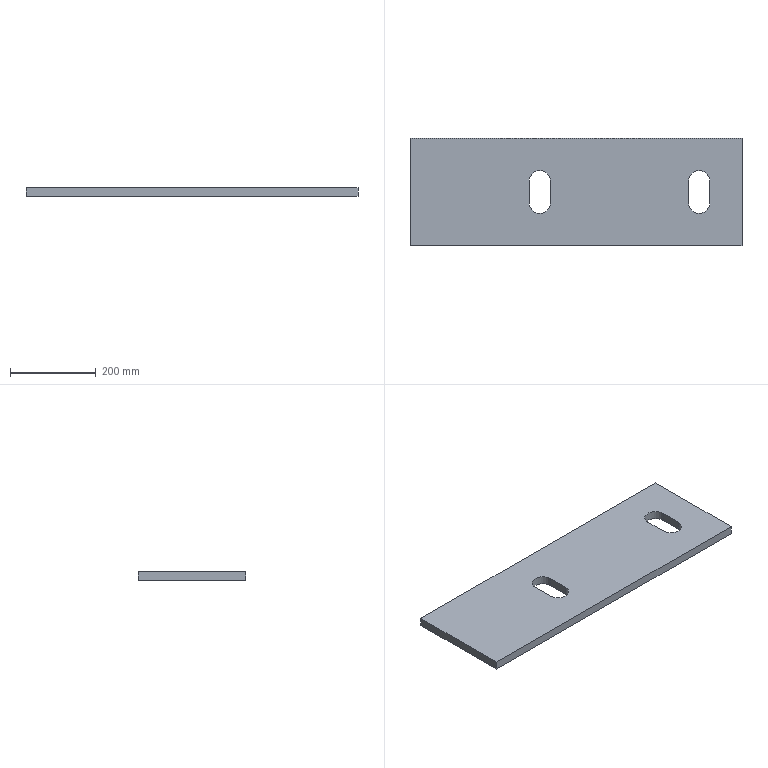Part | SolidWorks | features Extrusion 1 | 1 solid | 14 faces | box 775.098 x 250 x 20 mm | volume 3696953 mm3 | plane 10 | cylinder 4 | commonest cylinder face diameters 50 x4
STEP:
#1=CARTESIAN_POINT('',(13593.233,4558.16,20.));
#2=VERTEX_POINT('',#1);
#3=CARTESIAN_POINT('',(13543.233,4558.16,20.));
#4=VERTEX_POINT('',#3);
#5=CARTESIAN_POINT('',(13568.233,4558.16,20.));
#6=DIRECTION('',(0.,0.,1.));
#7=DIRECTION('',(1.,0.,0.));
#8=AXIS2_PLACEMENT_3D('',#5,#6,#7);
#9=CIRCLE('',#8,25.);
#10=EDGE_CURVE('',#2,#4,#9,.T.);
#11=ORIENTED_EDGE('',*,*,#10,.F.);
#12=CARTESIAN_POINT('',(13593.233,4508.16,20.));
#13=VERTEX_POINT('',#12);
#14=CARTESIAN_POINT('',(13593.233,4558.16,20.));
#15=DIRECTION('',(0.,1.,0.));
#16=VECTOR('',#15,1000.);
#17=LINE('',#14,#16);
#18=EDGE_CURVE('',#13,#2,#17,.T.);
#19=ORIENTED_EDGE('',*,*,#18,.F.);
#20=CARTESIAN_POINT('',(13543.233,4508.16,20.));
#21=VERTEX_POINT('',#20);
#22=CARTESIAN_POINT('',(13568.233,4508.16,20.));
#23=DIRECTION('',(0.,0.,1.));
#24=DIRECTION('',(1.,0.,0.));
#25=AXIS2_PLACEMENT_3D('',#22,#23,#24);
#26=CIRCLE('',#25,25.);
#27=EDGE_CURVE('',#21,#13,#26,.T.);
#28=ORIENTED_EDGE('',*,*,#27,.F.);
#29=CARTESIAN_POINT('',(13543.233,4558.16,20.));
#30=DIRECTION('',(0.,-1.,0.));
#31=VECTOR('',#30,1000.);
#32=LINE('',#29,#31);
#33=EDGE_CURVE('',#4,#21,#32,.T.);
#34=ORIENTED_EDGE('',*,*,#33,.F.);
#35=EDGE_LOOP('',(#11,#19,#28,#34));
#36=FACE_BOUND('',#35,.T.);
#37=CARTESIAN_POINT('',(14040.331,4658.16,20.));
#38=VERTEX_POINT('',#37);
#39=CARTESIAN_POINT('',(13265.233,4658.16,20.));
#40=VERTEX_POINT('',#39);
#41=CARTESIAN_POINT('',(13265.233,4658.16,20.));
#42=DIRECTION('',(-1.,0.,0.));
#43=VECTOR('',#42,1000.);
#44=LINE('',#41,#43);
#45=EDGE_CURVE('',#38,#40,#44,.T.);
#46=ORIENTED_EDGE('',*,*,#45,.T.);
#47=CARTESIAN_POINT('',(13265.233,4408.16,20.));
#48=VERTEX_POINT('',#47);
#49=CARTESIAN_POINT('',(13265.233,4658.16,20.));
#50=DIRECTION('',(0.,-1.,0.));
#51=VECTOR('',#50,1000.);
#52=LINE('',#49,#51);
#53=EDGE_CURVE('',#40,#48,#52,.T.);
#54=ORIENTED_EDGE('',*,*,#53,.T.);
#55=CARTESIAN_POINT('',(14040.331,4408.16,20.));
#56=VERTEX_POINT('',#55);
#57=CARTESIAN_POINT('',(13265.233,4408.16,20.));
#58=DIRECTION('',(1.,0.,0.));
#59=VECTOR('',#58,1000.);
#60=LINE('',#57,#59);
#61=EDGE_CURVE('',#48,#56,#60,.T.);
#62=ORIENTED_EDGE('',*,*,#61,.T.);
#63=CARTESIAN_POINT('',(14040.331,4658.16,20.));
#64=DIRECTION('',(0.,1.,0.));
#65=VECTOR('',#64,1000.);
#66=LINE('',#63,#65);
#67=EDGE_CURVE('',#56,#38,#66,.T.);
#68=ORIENTED_EDGE('',*,*,#67,.T.);
#69=EDGE_LOOP('',(#46,#54,#62,#68));
#70=FACE_OUTER_BOUND('',#69,.T.);
#71=CARTESIAN_POINT('',(13965.331,4558.16,20.));
#72=VERTEX_POINT('',#71);
#73=CARTESIAN_POINT('',(13915.331,4558.16,20.));
#74=VERTEX_POINT('',#73);
#75=CARTESIAN_POINT('',(13940.331,4558.16,20.));
#76=DIRECTION('',(0.,0.,1.));
#77=DIRECTION('',(1.,0.,0.));
#78=AXIS2_PLACEMENT_3D('',#75,#76,#77);
#79=CIRCLE('',#78,25.);
#80=EDGE_CURVE('',#72,#74,#79,.T.);
#81=ORIENTED_EDGE('',*,*,#80,.F.);
#82=CARTESIAN_POINT('',(13965.331,4508.16,20.));
#83=VERTEX_POINT('',#82);
#84=CARTESIAN_POINT('',(13965.331,4558.16,20.));
#85=DIRECTION('',(0.,1.,0.));
#86=VECTOR('',#85,1000.);
#87=LINE('',#84,#86);
#88=EDGE_CURVE('',#83,#72,#87,.T.);
#89=ORIENTED_EDGE('',*,*,#88,.F.);
#90=CARTESIAN_POINT('',(13915.331,4508.16,20.));
#91=VERTEX_POINT('',#90);
#92=CARTESIAN_POINT('',(13940.331,4508.16,20.));
#93=DIRECTION('',(0.,0.,1.));
#94=DIRECTION('',(1.,0.,0.));
#95=AXIS2_PLACEMENT_3D('',#92,#93,#94);
#96=CIRCLE('',#95,25.);
#97=EDGE_CURVE('',#91,#83,#96,.T.);
#98=ORIENTED_EDGE('',*,*,#97,.F.);
#99=CARTESIAN_POINT('',(13915.331,4558.16,20.));
#100=DIRECTION('',(0.,-1.,0.));
#101=VECTOR('',#100,1000.);
#102=LINE('',#99,#101);
#103=EDGE_CURVE('',#74,#91,#102,.T.);
#104=ORIENTED_EDGE('',*,*,#103,.F.);
#105=EDGE_LOOP('',(#81,#89,#98,#104));
#106=FACE_BOUND('',#105,.T.);
#107=CARTESIAN_POINT('',(0.,0.,20.));
#108=DIRECTION('',(0.,0.,-1.));
#109=DIRECTION('',(-1.,0.,0.));
#110=AXIS2_PLACEMENT_3D('',#107,#108,#109);
#111=PLANE('',#110);
#112=ADVANCED_FACE('',(#36,#70,#106),#111,.F.);
#113=CARTESIAN_POINT('',(14040.331,4658.16,0.));
#114=VERTEX_POINT('',#113);
#115=CARTESIAN_POINT('',(13265.233,4658.16,0.));
#116=VERTEX_POINT('',#115);
#117=CARTESIAN_POINT('',(13265.233,4658.16,0.));
#118=DIRECTION('',(-1.,0.,0.));
#119=VECTOR('',#118,1000.);
#120=LINE('',#117,#119);
#121=EDGE_CURVE('',#114,#116,#120,.T.);
#122=ORIENTED_EDGE('',*,*,#121,.F.);
#123=CARTESIAN_POINT('',(14040.331,4408.16,0.));
#124=VERTEX_POINT('',#123);
#125=CARTESIAN_POINT('',(14040.331,4658.16,0.));
#126=DIRECTION('',(0.,1.,0.));
#127=VECTOR('',#126,1000.);
#128=LINE('',#125,#127);
#129=EDGE_CURVE('',#124,#114,#128,.T.);
#130=ORIENTED_EDGE('',*,*,#129,.F.);
#131=CARTESIAN_POINT('',(13265.233,4408.16,0.));
#132=VERTEX_POINT('',#131);
#133=CARTESIAN_POINT('',(13265.233,4408.16,0.));
#134=DIRECTION('',(1.,0.,0.));
#135=VECTOR('',#134,1000.);
#136=LINE('',#133,#135);
#137=EDGE_CURVE('',#132,#124,#136,.T.);
#138=ORIENTED_EDGE('',*,*,#137,.F.);
#139=CARTESIAN_POINT('',(13265.233,4658.16,0.));
#140=DIRECTION('',(0.,-1.,0.));
#141=VECTOR('',#140,1000.);
#142=LINE('',#139,#141);
#143=EDGE_CURVE('',#116,#132,#142,.T.);
#144=ORIENTED_EDGE('',*,*,#143,.F.);
#145=EDGE_LOOP('',(#122,#130,#138,#144));
#146=FACE_OUTER_BOUND('',#145,.T.);
#147=CARTESIAN_POINT('',(13593.233,4508.16,0.));
#148=VERTEX_POINT('',#147);
#149=CARTESIAN_POINT('',(13593.233,4558.16,0.));
#150=VERTEX_POINT('',#149);
#151=CARTESIAN_POINT('',(13593.233,4558.16,0.));
#152=DIRECTION('',(0.,1.,0.));
#153=VECTOR('',#152,1000.);
#154=LINE('',#151,#153);
#155=EDGE_CURVE('',#148,#150,#154,.T.);
#156=ORIENTED_EDGE('',*,*,#155,.T.);
#157=CARTESIAN_POINT('',(13543.233,4558.16,0.));
#158=VERTEX_POINT('',#157);
#159=CARTESIAN_POINT('',(13568.233,4558.16,0.));
#160=DIRECTION('',(0.,0.,1.));
#161=DIRECTION('',(1.,0.,0.));
#162=AXIS2_PLACEMENT_3D('',#159,#160,#161);
#163=CIRCLE('',#162,25.);
#164=EDGE_CURVE('',#150,#158,#163,.T.);
#165=ORIENTED_EDGE('',*,*,#164,.T.);
#166=CARTESIAN_POINT('',(13543.233,4508.16,0.));
#167=VERTEX_POINT('',#166);
#168=CARTESIAN_POINT('',(13543.233,4558.16,0.));
#169=DIRECTION('',(0.,-1.,0.));
#170=VECTOR('',#169,1000.);
#171=LINE('',#168,#170);
#172=EDGE_CURVE('',#158,#167,#171,.T.);
#173=ORIENTED_EDGE('',*,*,#172,.T.);
#174=CARTESIAN_POINT('',(13568.233,4508.16,0.));
#175=DIRECTION('',(0.,0.,1.));
#176=DIRECTION('',(1.,0.,0.));
#177=AXIS2_PLACEMENT_3D('',#174,#175,#176);
#178=CIRCLE('',#177,25.);
#179=EDGE_CURVE('',#167,#148,#178,.T.);
#180=ORIENTED_EDGE('',*,*,#179,.T.);
#181=EDGE_LOOP('',(#156,#165,#173,#180));
#182=FACE_BOUND('',#181,.T.);
#183=CARTESIAN_POINT('',(13965.331,4508.16,0.));
#184=VERTEX_POINT('',#183);
#185=CARTESIAN_POINT('',(13965.331,4558.16,0.));
#186=VERTEX_POINT('',#185);
#187=CARTESIAN_POINT('',(13965.331,4558.16,0.));
#188=DIRECTION('',(0.,1.,0.));
#189=VECTOR('',#188,1000.);
#190=LINE('',#187,#189);
#191=EDGE_CURVE('',#184,#186,#190,.T.);
#192=ORIENTED_EDGE('',*,*,#191,.T.);
#193=CARTESIAN_POINT('',(13915.331,4558.16,0.));
#194=VERTEX_POINT('',#193);
#195=CARTESIAN_POINT('',(13940.331,4558.16,0.));
#196=DIRECTION('',(0.,0.,1.));
#197=DIRECTION('',(1.,0.,0.));
#198=AXIS2_PLACEMENT_3D('',#195,#196,#197);
#199=CIRCLE('',#198,25.);
#200=EDGE_CURVE('',#186,#194,#199,.T.);
#201=ORIENTED_EDGE('',*,*,#200,.T.);
#202=CARTESIAN_POINT('',(13915.331,4508.16,0.));
#203=VERTEX_POINT('',#202);
#204=CARTESIAN_POINT('',(13915.331,4558.16,0.));
#205=DIRECTION('',(0.,-1.,0.));
#206=VECTOR('',#205,1000.);
#207=LINE('',#204,#206);
#208=EDGE_CURVE('',#194,#203,#207,.T.);
#209=ORIENTED_EDGE('',*,*,#208,.T.);
#210=CARTESIAN_POINT('',(13940.331,4508.16,0.));
#211=DIRECTION('',(0.,0.,1.));
#212=DIRECTION('',(1.,0.,0.));
#213=AXIS2_PLACEMENT_3D('',#210,#211,#212);
#214=CIRCLE('',#213,25.);
#215=EDGE_CURVE('',#203,#184,#214,.T.);
#216=ORIENTED_EDGE('',*,*,#215,.T.);
#217=EDGE_LOOP('',(#192,#201,#209,#216));
#218=FACE_BOUND('',#217,.T.);
#219=CARTESIAN_POINT('',(0.,0.,0.));
#220=DIRECTION('',(0.,0.,-1.));
#221=DIRECTION('',(-1.,0.,0.));
#222=AXIS2_PLACEMENT_3D('',#219,#220,#221);
#223=PLANE('',#222);
#224=ADVANCED_FACE('',(#146,#182,#218),#223,.T.);
#225=ORIENTED_EDGE('',*,*,#121,.T.);
#226=CARTESIAN_POINT('',(13265.233,4658.16,20.));
#227=DIRECTION('',(0.,0.,-1.));
#228=VECTOR('',#227,1000.);
#229=LINE('',#226,#228);
#230=EDGE_CURVE('',#40,#116,#229,.T.);
#231=ORIENTED_EDGE('',*,*,#230,.F.);
#232=ORIENTED_EDGE('',*,*,#45,.F.);
#233=CARTESIAN_POINT('',(14040.331,4658.16,20.));
#234=DIRECTION('',(0.,0.,-1.));
#235=VECTOR('',#234,1000.);
#236=LINE('',#233,#235);
#237=EDGE_CURVE('',#38,#114,#236,.T.);
#238=ORIENTED_EDGE('',*,*,#237,.T.);
#239=EDGE_LOOP('',(#225,#231,#232,#238));
#240=FACE_OUTER_BOUND('',#239,.T.);
#241=CARTESIAN_POINT('',(13265.233,4658.16,20.));
#242=DIRECTION('',(0.,-1.,0.));
#243=DIRECTION('',(0.,0.,-1.));
#244=AXIS2_PLACEMENT_3D('',#241,#242,#243);
#245=PLANE('',#244);
#246=ADVANCED_FACE('',(#240),#245,.F.);
#247=ORIENTED_EDGE('',*,*,#143,.T.);
#248=CARTESIAN_POINT('',(13265.233,4408.16,20.));
#249=DIRECTION('',(0.,0.,-1.));
#250=VECTOR('',#249,1000.);
#251=LINE('',#248,#250);
#252=EDGE_CURVE('',#48,#132,#251,.T.);
#253=ORIENTED_EDGE('',*,*,#252,.F.);
#254=ORIENTED_EDGE('',*,*,#53,.F.);
#255=ORIENTED_EDGE('',*,*,#230,.T.);
#256=EDGE_LOOP('',(#247,#253,#254,#255));
#257=FACE_OUTER_BOUND('',#256,.T.);
#258=CARTESIAN_POINT('',(13265.233,4658.16,20.));
#259=DIRECTION('',(1.,0.,0.));
#260=DIRECTION('',(0.,1.,0.));
#261=AXIS2_PLACEMENT_3D('',#258,#259,#260);
#262=PLANE('',#261);
#263=ADVANCED_FACE('',(#257),#262,.F.);
#264=ORIENTED_EDGE('',*,*,#137,.T.);
#265=CARTESIAN_POINT('',(14040.331,4408.16,20.));
#266=DIRECTION('',(0.,0.,-1.));
#267=VECTOR('',#266,1000.);
#268=LINE('',#265,#267);
#269=EDGE_CURVE('',#56,#124,#268,.T.);
#270=ORIENTED_EDGE('',*,*,#269,.F.);
#271=ORIENTED_EDGE('',*,*,#61,.F.);
#272=ORIENTED_EDGE('',*,*,#252,.T.);
#273=EDGE_LOOP('',(#264,#270,#271,#272));
#274=FACE_OUTER_BOUND('',#273,.T.);
#275=CARTESIAN_POINT('',(13265.233,4408.16,20.));
#276=DIRECTION('',(0.,1.,0.));
#277=DIRECTION('',(0.,0.,1.));
#278=AXIS2_PLACEMENT_3D('',#275,#276,#277);
#279=PLANE('',#278);
#280=ADVANCED_FACE('',(#274),#279,.F.);
#281=ORIENTED_EDGE('',*,*,#129,.T.);
#282=ORIENTED_EDGE('',*,*,#237,.F.);
#283=ORIENTED_EDGE('',*,*,#67,.F.);
#284=ORIENTED_EDGE('',*,*,#269,.T.);
#285=EDGE_LOOP('',(#281,#282,#283,#284));
#286=FACE_OUTER_BOUND('',#285,.T.);
#287=CARTESIAN_POINT('',(14040.331,4658.16,20.));
#288=DIRECTION('',(-1.,0.,0.));
#289=DIRECTION('',(0.,0.,1.));
#290=AXIS2_PLACEMENT_3D('',#287,#288,#289);
#291=PLANE('',#290);
#292=ADVANCED_FACE('',(#286),#291,.F.);
#293=ORIENTED_EDGE('',*,*,#164,.F.);
#294=CARTESIAN_POINT('',(13593.233,4558.16,20.));
#295=DIRECTION('',(0.,0.,-1.));
#296=VECTOR('',#295,1000.);
#297=LINE('',#294,#296);
#298=EDGE_CURVE('',#2,#150,#297,.T.);
#299=ORIENTED_EDGE('',*,*,#298,.F.);
#300=ORIENTED_EDGE('',*,*,#10,.T.);
#301=CARTESIAN_POINT('',(13543.233,4558.16,20.));
#302=DIRECTION('',(0.,0.,-1.));
#303=VECTOR('',#302,1000.);
#304=LINE('',#301,#303);
#305=EDGE_CURVE('',#4,#158,#304,.T.);
#306=ORIENTED_EDGE('',*,*,#305,.T.);
#307=EDGE_LOOP('',(#293,#299,#300,#306));
#308=FACE_OUTER_BOUND('',#307,.T.);
#309=CARTESIAN_POINT('',(13568.233,4558.16,20.));
#310=DIRECTION('',(0.,0.,-1.));
#311=DIRECTION('',(-1.,0.,0.));
#312=AXIS2_PLACEMENT_3D('',#309,#310,#311);
#313=CYLINDRICAL_SURFACE('',#312,25.);
#314=ADVANCED_FACE('',(#308),#313,.F.);
#315=ORIENTED_EDGE('',*,*,#172,.F.);
#316=ORIENTED_EDGE('',*,*,#305,.F.);
#317=ORIENTED_EDGE('',*,*,#33,.T.);
#318=CARTESIAN_POINT('',(13543.233,4508.16,20.));
#319=DIRECTION('',(0.,0.,-1.));
#320=VECTOR('',#319,1000.);
#321=LINE('',#318,#320);
#322=EDGE_CURVE('',#21,#167,#321,.T.);
#323=ORIENTED_EDGE('',*,*,#322,.T.);
#324=EDGE_LOOP('',(#315,#316,#317,#323));
#325=FACE_OUTER_BOUND('',#324,.T.);
#326=CARTESIAN_POINT('',(13543.233,4558.16,20.));
#327=DIRECTION('',(1.,0.,0.));
#328=DIRECTION('',(0.,0.,-1.));
#329=AXIS2_PLACEMENT_3D('',#326,#327,#328);
#330=PLANE('',#329);
#331=ADVANCED_FACE('',(#325),#330,.T.);
#332=ORIENTED_EDGE('',*,*,#179,.F.);
#333=ORIENTED_EDGE('',*,*,#322,.F.);
#334=ORIENTED_EDGE('',*,*,#27,.T.);
#335=CARTESIAN_POINT('',(13593.233,4508.16,20.));
#336=DIRECTION('',(0.,0.,-1.));
#337=VECTOR('',#336,1000.);
#338=LINE('',#335,#337);
#339=EDGE_CURVE('',#13,#148,#338,.T.);
#340=ORIENTED_EDGE('',*,*,#339,.T.);
#341=EDGE_LOOP('',(#332,#333,#334,#340));
#342=FACE_OUTER_BOUND('',#341,.T.);
#343=CARTESIAN_POINT('',(13568.233,4508.16,20.));
#344=DIRECTION('',(0.,0.,-1.));
#345=DIRECTION('',(-1.,0.,0.));
#346=AXIS2_PLACEMENT_3D('',#343,#344,#345);
#347=CYLINDRICAL_SURFACE('',#346,25.);
#348=ADVANCED_FACE('',(#342),#347,.F.);
#349=ORIENTED_EDGE('',*,*,#155,.F.);
#350=ORIENTED_EDGE('',*,*,#339,.F.);
#351=ORIENTED_EDGE('',*,*,#18,.T.);
#352=ORIENTED_EDGE('',*,*,#298,.T.);
#353=EDGE_LOOP('',(#349,#350,#351,#352));
#354=FACE_OUTER_BOUND('',#353,.T.);
#355=CARTESIAN_POINT('',(13593.233,4558.16,20.));
#356=DIRECTION('',(-1.,0.,0.));
#357=DIRECTION('',(0.,0.,1.));
#358=AXIS2_PLACEMENT_3D('',#355,#356,#357);
#359=PLANE('',#358);
#360=ADVANCED_FACE('',(#354),#359,.T.);
#361=ORIENTED_EDGE('',*,*,#200,.F.);
#362=CARTESIAN_POINT('',(13965.331,4558.16,20.));
#363=DIRECTION('',(0.,0.,-1.));
#364=VECTOR('',#363,1000.);
#365=LINE('',#362,#364);
#366=EDGE_CURVE('',#72,#186,#365,.T.);
#367=ORIENTED_EDGE('',*,*,#366,.F.);
#368=ORIENTED_EDGE('',*,*,#80,.T.);
#369=CARTESIAN_POINT('',(13915.331,4558.16,20.));
#370=DIRECTION('',(0.,0.,-1.));
#371=VECTOR('',#370,1000.);
#372=LINE('',#369,#371);
#373=EDGE_CURVE('',#74,#194,#372,.T.);
#374=ORIENTED_EDGE('',*,*,#373,.T.);
#375=EDGE_LOOP('',(#361,#367,#368,#374));
#376=FACE_OUTER_BOUND('',#375,.T.);
#377=CARTESIAN_POINT('',(13940.331,4558.16,20.));
#378=DIRECTION('',(0.,0.,-1.));
#379=DIRECTION('',(-1.,0.,0.));
#380=AXIS2_PLACEMENT_3D('',#377,#378,#379);
#381=CYLINDRICAL_SURFACE('',#380,25.);
#382=ADVANCED_FACE('',(#376),#381,.F.);
#383=ORIENTED_EDGE('',*,*,#208,.F.);
#384=ORIENTED_EDGE('',*,*,#373,.F.);
#385=ORIENTED_EDGE('',*,*,#103,.T.);
#386=CARTESIAN_POINT('',(13915.331,4508.16,20.));
#387=DIRECTION('',(0.,0.,-1.));
#388=VECTOR('',#387,1000.);
#389=LINE('',#386,#388);
#390=EDGE_CURVE('',#91,#203,#389,.T.);
#391=ORIENTED_EDGE('',*,*,#390,.T.);
#392=EDGE_LOOP('',(#383,#384,#385,#391));
#393=FACE_OUTER_BOUND('',#392,.T.);
#394=CARTESIAN_POINT('',(13915.331,4558.16,20.));
#395=DIRECTION('',(1.,0.,0.));
#396=DIRECTION('',(0.,0.,-1.));
#397=AXIS2_PLACEMENT_3D('',#394,#395,#396);
#398=PLANE('',#397);
#399=ADVANCED_FACE('',(#393),#398,.T.);
#400=ORIENTED_EDGE('',*,*,#215,.F.);
#401=ORIENTED_EDGE('',*,*,#390,.F.);
#402=ORIENTED_EDGE('',*,*,#97,.T.);
#403=CARTESIAN_POINT('',(13965.331,4508.16,20.));
#404=DIRECTION('',(0.,0.,-1.));
#405=VECTOR('',#404,1000.);
#406=LINE('',#403,#405);
#407=EDGE_CURVE('',#83,#184,#406,.T.);
#408=ORIENTED_EDGE('',*,*,#407,.T.);
#409=EDGE_LOOP('',(#400,#401,#402,#408));
#410=FACE_OUTER_BOUND('',#409,.T.);
#411=CARTESIAN_POINT('',(13940.331,4508.16,20.));
#412=DIRECTION('',(0.,0.,-1.));
#413=DIRECTION('',(-1.,0.,0.));
#414=AXIS2_PLACEMENT_3D('',#411,#412,#413);
#415=CYLINDRICAL_SURFACE('',#414,25.);
#416=ADVANCED_FACE('',(#410),#415,.F.);
#417=ORIENTED_EDGE('',*,*,#191,.F.);
#418=ORIENTED_EDGE('',*,*,#407,.F.);
#419=ORIENTED_EDGE('',*,*,#88,.T.);
#420=ORIENTED_EDGE('',*,*,#366,.T.);
#421=EDGE_LOOP('',(#417,#418,#419,#420));
#422=FACE_OUTER_BOUND('',#421,.T.);
#423=CARTESIAN_POINT('',(13965.331,4558.16,20.));
#424=DIRECTION('',(-1.,0.,0.));
#425=DIRECTION('',(0.,0.,1.));
#426=AXIS2_PLACEMENT_3D('',#423,#424,#425);
#427=PLANE('',#426);
#428=ADVANCED_FACE('',(#422),#427,.T.);
#429=CLOSED_SHELL('',(#112,#224,#246,#263,#280,#292,#314,#331,#348,#360,#382,#399,#416,#428));
#430=MANIFOLD_SOLID_BREP('',#429);
#431=CARTESIAN_POINT('',(0.,0.,0.));
#432=DIRECTION('',(0.,0.,1.));
#433=DIRECTION('',(1.,0.,0.));
#434=AXIS2_PLACEMENT_3D('',#431,#432,#433);
#435=(LENGTH_UNIT()NAMED_UNIT(*)SI_UNIT(.MILLI.,.METRE.));
#436=UNCERTAINTY_MEASURE_WITH_UNIT(LENGTH_MEASURE(0.00001),#435,'','');
#437=(NAMED_UNIT(*)PLANE_ANGLE_UNIT()SI_UNIT($,.RADIAN.));
#438=(NAMED_UNIT(*)SI_UNIT($,.STERADIAN.)SOLID_ANGLE_UNIT());
#439=(GEOMETRIC_REPRESENTATION_CONTEXT(3)GLOBAL_UNCERTAINTY_ASSIGNED_CONTEXT((#436))GLOBAL_UNIT_ASSIGNED_CONTEXT((#435,#437,#438))REPRESENTATION_CONTEXT('',''));
#440=ADVANCED_BREP_SHAPE_REPRESENTATION('',(#430,#434),#439);